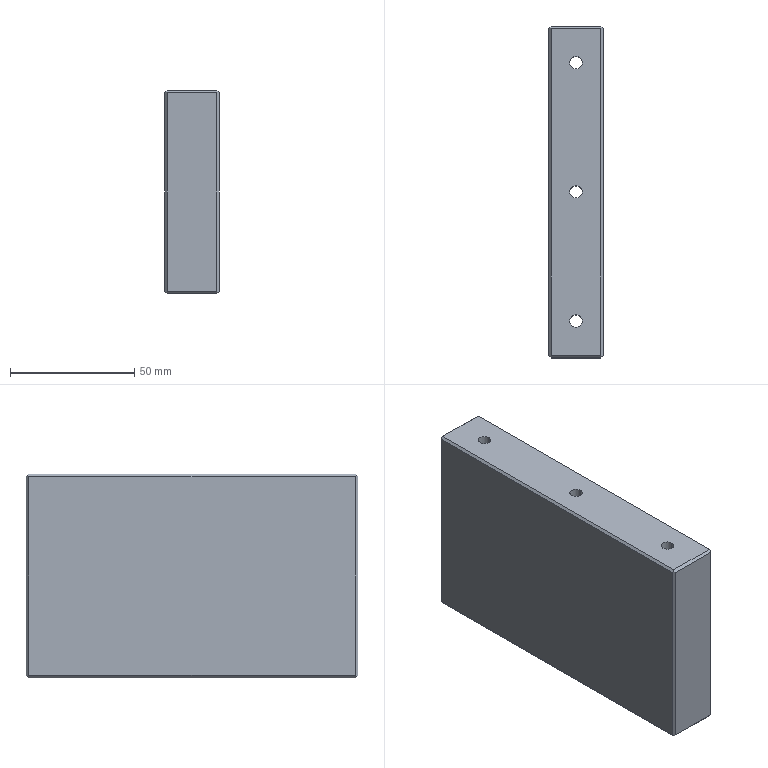Part | Creo | features DATUM PLANE 3, CHAMFER 1, COORDINATE SYSTEM 1, CURVE 1, PROTRUSION 1 | 1 solid | 24 faces | box 22 x 133.5 x 82 mm | volume 235535 mm3 | plane 18 | cylinder 6 | commonest cylinder face diameters 5 x6
STEP:
#1=CARTESIAN_POINT('',(0.,0.,0.));
#2=DIRECTION('',(0.,0.,1.));
#3=DIRECTION('',(1.,0.,0.));
#4=AXIS2_PLACEMENT_3D('',#1,#2,#3);
#5=CARTESIAN_POINT('',(-10.,-65.75,0.));
#6=VERTEX_POINT('',#5);
#7=CARTESIAN_POINT('',(-10.,65.75,0.));
#8=VERTEX_POINT('',#7);
#9=CARTESIAN_POINT('',(-10.,-65.75,0.));
#10=DIRECTION('',(0.,1.,0.));
#11=VECTOR('',#10,131.5);
#12=LINE('',#9,#11);
#13=EDGE_CURVE('',#6,#8,#12,.T.);
#14=ORIENTED_EDGE('',*,*,#13,.F.);
#15=CARTESIAN_POINT('',(10.,-65.75,0.));
#16=VERTEX_POINT('',#15);
#17=CARTESIAN_POINT('',(10.,-65.75,0.));
#18=DIRECTION('',(-1.,0.,0.));
#19=VECTOR('',#18,20.);
#20=LINE('',#17,#19);
#21=EDGE_CURVE('',#16,#6,#20,.T.);
#22=ORIENTED_EDGE('',*,*,#21,.F.);
#23=CARTESIAN_POINT('',(10.,65.75,0.));
#24=VERTEX_POINT('',#23);
#25=CARTESIAN_POINT('',(10.,65.75,0.));
#26=DIRECTION('',(0.,-1.,0.));
#27=VECTOR('',#26,131.5);
#28=LINE('',#25,#27);
#29=EDGE_CURVE('',#24,#16,#28,.T.);
#30=ORIENTED_EDGE('',*,*,#29,.F.);
#31=CARTESIAN_POINT('',(-10.,65.75,0.));
#32=DIRECTION('',(1.,0.,0.));
#33=VECTOR('',#32,20.);
#34=LINE('',#31,#33);
#35=EDGE_CURVE('',#8,#24,#34,.T.);
#36=ORIENTED_EDGE('',*,*,#35,.F.);
#37=EDGE_LOOP('',(#14,#22,#30,#36));
#38=FACE_OUTER_BOUND('',#37,.F.);
#39=CARTESIAN_POINT('',(2.5,0.,0.));
#40=VERTEX_POINT('',#39);
#41=CARTESIAN_POINT('',(-2.5,0.,0.));
#42=VERTEX_POINT('',#41);
#43=CARTESIAN_POINT('',(0.,0.,0.));
#44=DIRECTION('',(0.,0.,-1.));
#45=DIRECTION('',(1.,0.,0.));
#46=AXIS2_PLACEMENT_3D('',#43,#44,#45);
#47=CIRCLE('',#46,2.5);
#48=EDGE_CURVE('',#40,#42,#47,.T.);
#49=ORIENTED_EDGE('',*,*,#48,.T.);
#50=CARTESIAN_POINT('',(0.,0.,0.));
#51=DIRECTION('',(0.,0.,-1.));
#52=DIRECTION('',(-1.,0.,0.));
#53=AXIS2_PLACEMENT_3D('',#50,#51,#52);
#54=CIRCLE('',#53,2.5);
#55=EDGE_CURVE('',#42,#40,#54,.T.);
#56=ORIENTED_EDGE('',*,*,#55,.T.);
#57=EDGE_LOOP('',(#49,#56));
#58=FACE_BOUND('',#57,.F.);
#59=CARTESIAN_POINT('',(2.5,-52.,0.));
#60=VERTEX_POINT('',#59);
#61=CARTESIAN_POINT('',(-2.5,-52.,0.));
#62=VERTEX_POINT('',#61);
#63=CARTESIAN_POINT('',(0.,-52.,0.));
#64=DIRECTION('',(0.,0.,-1.));
#65=DIRECTION('',(1.,0.,0.));
#66=AXIS2_PLACEMENT_3D('',#63,#64,#65);
#67=CIRCLE('',#66,2.5);
#68=EDGE_CURVE('',#60,#62,#67,.T.);
#69=ORIENTED_EDGE('',*,*,#68,.T.);
#70=CARTESIAN_POINT('',(0.,-52.,0.));
#71=DIRECTION('',(0.,0.,-1.));
#72=DIRECTION('',(-1.,0.,0.));
#73=AXIS2_PLACEMENT_3D('',#70,#71,#72);
#74=CIRCLE('',#73,2.5);
#75=EDGE_CURVE('',#62,#60,#74,.T.);
#76=ORIENTED_EDGE('',*,*,#75,.T.);
#77=EDGE_LOOP('',(#69,#76));
#78=FACE_BOUND('',#77,.F.);
#79=CARTESIAN_POINT('',(2.5,52.,0.));
#80=VERTEX_POINT('',#79);
#81=CARTESIAN_POINT('',(-2.5,52.,0.));
#82=VERTEX_POINT('',#81);
#83=CARTESIAN_POINT('',(0.,52.,0.));
#84=DIRECTION('',(0.,0.,-1.));
#85=DIRECTION('',(1.,0.,0.));
#86=AXIS2_PLACEMENT_3D('',#83,#84,#85);
#87=CIRCLE('',#86,2.5);
#88=EDGE_CURVE('',#80,#82,#87,.T.);
#89=ORIENTED_EDGE('',*,*,#88,.T.);
#90=CARTESIAN_POINT('',(0.,52.,0.));
#91=DIRECTION('',(0.,0.,-1.));
#92=DIRECTION('',(-1.,0.,0.));
#93=AXIS2_PLACEMENT_3D('',#90,#91,#92);
#94=CIRCLE('',#93,2.5);
#95=EDGE_CURVE('',#82,#80,#94,.T.);
#96=ORIENTED_EDGE('',*,*,#95,.T.);
#97=EDGE_LOOP('',(#89,#96));
#98=FACE_BOUND('',#97,.F.);
#99=CARTESIAN_POINT('',(0.,0.,0.));
#100=DIRECTION('',(0.,0.,1.));
#101=DIRECTION('',(1.,0.,0.));
#102=AXIS2_PLACEMENT_3D('',#99,#100,#101);
#103=PLANE('',#102);
#104=ADVANCED_FACE('',(#38,#58,#78,#98),#103,.F.);
#105=ORIENTED_EDGE('',*,*,#88,.F.);
#106=CARTESIAN_POINT('',(2.5,52.,82.));
#107=VERTEX_POINT('',#106);
#108=CARTESIAN_POINT('',(2.5,52.,0.));
#109=DIRECTION('',(0.,0.,1.));
#110=VECTOR('',#109,82.);
#111=LINE('',#108,#110);
#112=EDGE_CURVE('',#80,#107,#111,.T.);
#113=ORIENTED_EDGE('',*,*,#112,.T.);
#114=CARTESIAN_POINT('',(-2.5,52.,82.));
#115=VERTEX_POINT('',#114);
#116=CARTESIAN_POINT('',(0.,52.,82.));
#117=DIRECTION('',(0.,0.,-1.));
#118=DIRECTION('',(1.,0.,0.));
#119=AXIS2_PLACEMENT_3D('',#116,#117,#118);
#120=CIRCLE('',#119,2.5);
#121=EDGE_CURVE('',#107,#115,#120,.T.);
#122=ORIENTED_EDGE('',*,*,#121,.T.);
#123=CARTESIAN_POINT('',(-2.5,52.,0.));
#124=DIRECTION('',(0.,0.,1.));
#125=VECTOR('',#124,82.);
#126=LINE('',#123,#125);
#127=EDGE_CURVE('',#82,#115,#126,.T.);
#128=ORIENTED_EDGE('',*,*,#127,.F.);
#129=EDGE_LOOP('',(#105,#113,#122,#128));
#130=FACE_OUTER_BOUND('',#129,.F.);
#131=CARTESIAN_POINT('',(0.,52.,0.));
#132=DIRECTION('',(0.,0.,1.));
#133=DIRECTION('',(1.,0.,0.));
#134=AXIS2_PLACEMENT_3D('',#131,#132,#133);
#135=CYLINDRICAL_SURFACE('',#134,2.5);
#136=ADVANCED_FACE('',(#130),#135,.F.);
#137=ORIENTED_EDGE('',*,*,#95,.F.);
#138=ORIENTED_EDGE('',*,*,#127,.T.);
#139=CARTESIAN_POINT('',(0.,52.,82.));
#140=DIRECTION('',(0.,0.,-1.));
#141=DIRECTION('',(-1.,0.,0.));
#142=AXIS2_PLACEMENT_3D('',#139,#140,#141);
#143=CIRCLE('',#142,2.5);
#144=EDGE_CURVE('',#115,#107,#143,.T.);
#145=ORIENTED_EDGE('',*,*,#144,.T.);
#146=ORIENTED_EDGE('',*,*,#112,.F.);
#147=EDGE_LOOP('',(#137,#138,#145,#146));
#148=FACE_OUTER_BOUND('',#147,.F.);
#149=CARTESIAN_POINT('',(0.,52.,0.));
#150=DIRECTION('',(0.,0.,1.));
#151=DIRECTION('',(1.,0.,0.));
#152=AXIS2_PLACEMENT_3D('',#149,#150,#151);
#153=CYLINDRICAL_SURFACE('',#152,2.5);
#154=ADVANCED_FACE('',(#148),#153,.F.);
#155=CARTESIAN_POINT('',(10.,65.75,82.));
#156=VERTEX_POINT('',#155);
#157=CARTESIAN_POINT('',(-10.,65.75,82.));
#158=VERTEX_POINT('',#157);
#159=CARTESIAN_POINT('',(10.,65.75,82.));
#160=DIRECTION('',(-1.,0.,0.));
#161=VECTOR('',#160,20.);
#162=LINE('',#159,#161);
#163=EDGE_CURVE('',#156,#158,#162,.T.);
#164=ORIENTED_EDGE('',*,*,#163,.F.);
#165=CARTESIAN_POINT('',(10.,-65.75,82.));
#166=VERTEX_POINT('',#165);
#167=CARTESIAN_POINT('',(10.,-65.75,82.));
#168=DIRECTION('',(0.,1.,0.));
#169=VECTOR('',#168,131.5);
#170=LINE('',#167,#169);
#171=EDGE_CURVE('',#166,#156,#170,.T.);
#172=ORIENTED_EDGE('',*,*,#171,.F.);
#173=CARTESIAN_POINT('',(-10.,-65.75,82.));
#174=VERTEX_POINT('',#173);
#175=CARTESIAN_POINT('',(-10.,-65.75,82.));
#176=DIRECTION('',(1.,0.,0.));
#177=VECTOR('',#176,20.);
#178=LINE('',#175,#177);
#179=EDGE_CURVE('',#174,#166,#178,.T.);
#180=ORIENTED_EDGE('',*,*,#179,.F.);
#181=CARTESIAN_POINT('',(-10.,65.75,82.));
#182=DIRECTION('',(0.,-1.,0.));
#183=VECTOR('',#182,131.5);
#184=LINE('',#181,#183);
#185=EDGE_CURVE('',#158,#174,#184,.T.);
#186=ORIENTED_EDGE('',*,*,#185,.F.);
#187=EDGE_LOOP('',(#164,#172,#180,#186));
#188=FACE_OUTER_BOUND('',#187,.F.);
#189=CARTESIAN_POINT('',(2.5,0.,82.));
#190=VERTEX_POINT('',#189);
#191=CARTESIAN_POINT('',(-2.5,0.,82.));
#192=VERTEX_POINT('',#191);
#193=CARTESIAN_POINT('',(0.,0.,82.));
#194=DIRECTION('',(0.,0.,-1.));
#195=DIRECTION('',(1.,0.,0.));
#196=AXIS2_PLACEMENT_3D('',#193,#194,#195);
#197=CIRCLE('',#196,2.5);
#198=EDGE_CURVE('',#190,#192,#197,.T.);
#199=ORIENTED_EDGE('',*,*,#198,.F.);
#200=CARTESIAN_POINT('',(0.,0.,82.));
#201=DIRECTION('',(0.,0.,-1.));
#202=DIRECTION('',(-1.,0.,0.));
#203=AXIS2_PLACEMENT_3D('',#200,#201,#202);
#204=CIRCLE('',#203,2.5);
#205=EDGE_CURVE('',#192,#190,#204,.T.);
#206=ORIENTED_EDGE('',*,*,#205,.F.);
#207=EDGE_LOOP('',(#199,#206));
#208=FACE_BOUND('',#207,.F.);
#209=CARTESIAN_POINT('',(2.5,-52.,82.));
#210=VERTEX_POINT('',#209);
#211=CARTESIAN_POINT('',(-2.5,-52.,82.));
#212=VERTEX_POINT('',#211);
#213=CARTESIAN_POINT('',(0.,-52.,82.));
#214=DIRECTION('',(0.,0.,-1.));
#215=DIRECTION('',(1.,0.,0.));
#216=AXIS2_PLACEMENT_3D('',#213,#214,#215);
#217=CIRCLE('',#216,2.5);
#218=EDGE_CURVE('',#210,#212,#217,.T.);
#219=ORIENTED_EDGE('',*,*,#218,.F.);
#220=CARTESIAN_POINT('',(0.,-52.,82.));
#221=DIRECTION('',(0.,0.,-1.));
#222=DIRECTION('',(-1.,0.,0.));
#223=AXIS2_PLACEMENT_3D('',#220,#221,#222);
#224=CIRCLE('',#223,2.5);
#225=EDGE_CURVE('',#212,#210,#224,.T.);
#226=ORIENTED_EDGE('',*,*,#225,.F.);
#227=EDGE_LOOP('',(#219,#226));
#228=FACE_BOUND('',#227,.F.);
#229=ORIENTED_EDGE('',*,*,#121,.F.);
#230=ORIENTED_EDGE('',*,*,#144,.F.);
#231=EDGE_LOOP('',(#229,#230));
#232=FACE_BOUND('',#231,.F.);
#233=CARTESIAN_POINT('',(0.,0.,82.));
#234=DIRECTION('',(0.,0.,1.));
#235=DIRECTION('',(1.,0.,0.));
#236=AXIS2_PLACEMENT_3D('',#233,#234,#235);
#237=PLANE('',#236);
#238=ADVANCED_FACE('',(#188,#208,#228,#232),#237,.T.);
#239=ORIENTED_EDGE('',*,*,#48,.F.);
#240=CARTESIAN_POINT('',(2.5,0.,0.));
#241=DIRECTION('',(0.,0.,1.));
#242=VECTOR('',#241,82.);
#243=LINE('',#240,#242);
#244=EDGE_CURVE('',#40,#190,#243,.T.);
#245=ORIENTED_EDGE('',*,*,#244,.T.);
#246=ORIENTED_EDGE('',*,*,#198,.T.);
#247=CARTESIAN_POINT('',(-2.5,0.,0.));
#248=DIRECTION('',(0.,0.,1.));
#249=VECTOR('',#248,82.);
#250=LINE('',#247,#249);
#251=EDGE_CURVE('',#42,#192,#250,.T.);
#252=ORIENTED_EDGE('',*,*,#251,.F.);
#253=EDGE_LOOP('',(#239,#245,#246,#252));
#254=FACE_OUTER_BOUND('',#253,.F.);
#255=CARTESIAN_POINT('',(0.,0.,0.));
#256=DIRECTION('',(0.,0.,1.));
#257=DIRECTION('',(1.,0.,0.));
#258=AXIS2_PLACEMENT_3D('',#255,#256,#257);
#259=CYLINDRICAL_SURFACE('',#258,2.5);
#260=ADVANCED_FACE('',(#254),#259,.F.);
#261=ORIENTED_EDGE('',*,*,#55,.F.);
#262=ORIENTED_EDGE('',*,*,#251,.T.);
#263=ORIENTED_EDGE('',*,*,#205,.T.);
#264=ORIENTED_EDGE('',*,*,#244,.F.);
#265=EDGE_LOOP('',(#261,#262,#263,#264));
#266=FACE_OUTER_BOUND('',#265,.F.);
#267=CARTESIAN_POINT('',(0.,0.,0.));
#268=DIRECTION('',(0.,0.,1.));
#269=DIRECTION('',(1.,0.,0.));
#270=AXIS2_PLACEMENT_3D('',#267,#268,#269);
#271=CYLINDRICAL_SURFACE('',#270,2.5);
#272=ADVANCED_FACE('',(#266),#271,.F.);
#273=ORIENTED_EDGE('',*,*,#68,.F.);
#274=CARTESIAN_POINT('',(2.5,-52.,0.));
#275=DIRECTION('',(0.,0.,1.));
#276=VECTOR('',#275,82.);
#277=LINE('',#274,#276);
#278=EDGE_CURVE('',#60,#210,#277,.T.);
#279=ORIENTED_EDGE('',*,*,#278,.T.);
#280=ORIENTED_EDGE('',*,*,#218,.T.);
#281=CARTESIAN_POINT('',(-2.5,-52.,0.));
#282=DIRECTION('',(0.,0.,1.));
#283=VECTOR('',#282,82.);
#284=LINE('',#281,#283);
#285=EDGE_CURVE('',#62,#212,#284,.T.);
#286=ORIENTED_EDGE('',*,*,#285,.F.);
#287=EDGE_LOOP('',(#273,#279,#280,#286));
#288=FACE_OUTER_BOUND('',#287,.F.);
#289=CARTESIAN_POINT('',(0.,-52.,0.));
#290=DIRECTION('',(0.,0.,1.));
#291=DIRECTION('',(1.,0.,0.));
#292=AXIS2_PLACEMENT_3D('',#289,#290,#291);
#293=CYLINDRICAL_SURFACE('',#292,2.5);
#294=ADVANCED_FACE('',(#288),#293,.F.);
#295=ORIENTED_EDGE('',*,*,#75,.F.);
#296=ORIENTED_EDGE('',*,*,#285,.T.);
#297=ORIENTED_EDGE('',*,*,#225,.T.);
#298=ORIENTED_EDGE('',*,*,#278,.F.);
#299=EDGE_LOOP('',(#295,#296,#297,#298));
#300=FACE_OUTER_BOUND('',#299,.F.);
#301=CARTESIAN_POINT('',(0.,-52.,0.));
#302=DIRECTION('',(0.,0.,1.));
#303=DIRECTION('',(1.,0.,0.));
#304=AXIS2_PLACEMENT_3D('',#301,#302,#303);
#305=CYLINDRICAL_SURFACE('',#304,2.5);
#306=ADVANCED_FACE('',(#300),#305,.F.);
#307=CARTESIAN_POINT('',(10.,66.75,81.));
#308=VERTEX_POINT('',#307);
#309=CARTESIAN_POINT('',(-10.,66.75,81.));
#310=VERTEX_POINT('',#309);
#311=CARTESIAN_POINT('',(10.,66.75,81.));
#312=DIRECTION('',(-1.,0.,0.));
#313=VECTOR('',#312,20.);
#314=LINE('',#311,#313);
#315=EDGE_CURVE('',#308,#310,#314,.T.);
#316=ORIENTED_EDGE('',*,*,#315,.F.);
#317=CARTESIAN_POINT('',(10.5,66.25,81.5));
#318=VERTEX_POINT('',#317);
#319=CARTESIAN_POINT('',(10.,66.75,81.));
#320=DIRECTION('',(0.5774,-0.5774,0.5774));
#321=VECTOR('',#320,0.866);
#322=LINE('',#319,#321);
#323=EDGE_CURVE('',#308,#318,#322,.T.);
#324=ORIENTED_EDGE('',*,*,#323,.T.);
#325=CARTESIAN_POINT('',(10.,65.75,82.));
#326=DIRECTION('',(0.5774,0.5774,-0.5774));
#327=VECTOR('',#326,0.866);
#328=LINE('',#325,#327);
#329=EDGE_CURVE('',#156,#318,#328,.T.);
#330=ORIENTED_EDGE('',*,*,#329,.F.);
#331=ORIENTED_EDGE('',*,*,#163,.T.);
#332=CARTESIAN_POINT('',(-10.5,66.25,81.5));
#333=VERTEX_POINT('',#332);
#334=CARTESIAN_POINT('',(-10.,65.75,82.));
#335=DIRECTION('',(-0.5774,0.5774,-0.5774));
#336=VECTOR('',#335,0.866);
#337=LINE('',#334,#336);
#338=EDGE_CURVE('',#158,#333,#337,.T.);
#339=ORIENTED_EDGE('',*,*,#338,.T.);
#340=CARTESIAN_POINT('',(-10.5,66.25,81.5));
#341=DIRECTION('',(0.5774,0.5774,-0.5774));
#342=VECTOR('',#341,0.866);
#343=LINE('',#340,#342);
#344=EDGE_CURVE('',#333,#310,#343,.T.);
#345=ORIENTED_EDGE('',*,*,#344,.T.);
#346=EDGE_LOOP('',(#316,#324,#330,#331,#339,#345));
#347=FACE_OUTER_BOUND('',#346,.F.);
#348=CARTESIAN_POINT('',(0.,66.25,81.5));
#349=DIRECTION('',(0.,0.7071,0.7071));
#350=DIRECTION('',(0.,0.7071,-0.7071));
#351=AXIS2_PLACEMENT_3D('',#348,#349,#350);
#352=PLANE('',#351);
#353=ADVANCED_FACE('',(#347),#352,.T.);
#354=CARTESIAN_POINT('',(10.,66.75,1.));
#355=VERTEX_POINT('',#354);
#356=CARTESIAN_POINT('',(10.,66.75,81.));
#357=DIRECTION('',(0.,0.,-1.));
#358=VECTOR('',#357,80.);
#359=LINE('',#356,#358);
#360=EDGE_CURVE('',#308,#355,#359,.T.);
#361=ORIENTED_EDGE('',*,*,#360,.F.);
#362=ORIENTED_EDGE('',*,*,#315,.T.);
#363=CARTESIAN_POINT('',(-10.,66.75,1.));
#364=VERTEX_POINT('',#363);
#365=CARTESIAN_POINT('',(-10.,66.75,81.));
#366=DIRECTION('',(0.,0.,-1.));
#367=VECTOR('',#366,80.);
#368=LINE('',#365,#367);
#369=EDGE_CURVE('',#310,#364,#368,.T.);
#370=ORIENTED_EDGE('',*,*,#369,.T.);
#371=CARTESIAN_POINT('',(-10.,66.75,1.));
#372=DIRECTION('',(1.,0.,0.));
#373=VECTOR('',#372,20.);
#374=LINE('',#371,#373);
#375=EDGE_CURVE('',#364,#355,#374,.T.);
#376=ORIENTED_EDGE('',*,*,#375,.T.);
#377=EDGE_LOOP('',(#361,#362,#370,#376));
#378=FACE_OUTER_BOUND('',#377,.F.);
#379=CARTESIAN_POINT('',(11.,66.75,0.));
#380=DIRECTION('',(0.,1.,0.));
#381=DIRECTION('',(-1.,0.,0.));
#382=AXIS2_PLACEMENT_3D('',#379,#380,#381);
#383=PLANE('',#382);
#384=ADVANCED_FACE('',(#378),#383,.T.);
#385=ORIENTED_EDGE('',*,*,#360,.T.);
#386=CARTESIAN_POINT('',(10.5,66.25,0.5));
#387=VERTEX_POINT('',#386);
#388=CARTESIAN_POINT('',(10.,66.75,1.));
#389=DIRECTION('',(0.5774,-0.5774,-0.5774));
#390=VECTOR('',#389,0.866);
#391=LINE('',#388,#390);
#392=EDGE_CURVE('',#355,#387,#391,.T.);
#393=ORIENTED_EDGE('',*,*,#392,.T.);
#394=CARTESIAN_POINT('',(11.,65.75,1.));
#395=VERTEX_POINT('',#394);
#396=CARTESIAN_POINT('',(11.,65.75,1.));
#397=DIRECTION('',(-0.5774,0.5774,-0.5774));
#398=VECTOR('',#397,0.866);
#399=LINE('',#396,#398);
#400=EDGE_CURVE('',#395,#387,#399,.T.);
#401=ORIENTED_EDGE('',*,*,#400,.F.);
#402=CARTESIAN_POINT('',(11.,65.75,81.));
#403=VERTEX_POINT('',#402);
#404=CARTESIAN_POINT('',(11.,65.75,81.));
#405=DIRECTION('',(0.,0.,-1.));
#406=VECTOR('',#405,80.);
#407=LINE('',#404,#406);
#408=EDGE_CURVE('',#403,#395,#407,.T.);
#409=ORIENTED_EDGE('',*,*,#408,.F.);
#410=CARTESIAN_POINT('',(10.5,66.25,81.5));
#411=DIRECTION('',(0.5774,-0.5774,-0.5774));
#412=VECTOR('',#411,0.866);
#413=LINE('',#410,#412);
#414=EDGE_CURVE('',#318,#403,#413,.T.);
#415=ORIENTED_EDGE('',*,*,#414,.F.);
#416=ORIENTED_EDGE('',*,*,#323,.F.);
#417=EDGE_LOOP('',(#385,#393,#401,#409,#415,#416));
#418=FACE_OUTER_BOUND('',#417,.F.);
#419=CARTESIAN_POINT('',(10.5,66.25,41.));
#420=DIRECTION('',(0.7071,0.7071,0.));
#421=DIRECTION('',(0.7071,-0.7071,0.));
#422=AXIS2_PLACEMENT_3D('',#419,#420,#421);
#423=PLANE('',#422);
#424=ADVANCED_FACE('',(#418),#423,.T.);
#425=ORIENTED_EDGE('',*,*,#35,.T.);
#426=CARTESIAN_POINT('',(10.5,66.25,0.5));
#427=DIRECTION('',(-0.5774,-0.5774,-0.5774));
#428=VECTOR('',#427,0.866);
#429=LINE('',#426,#428);
#430=EDGE_CURVE('',#387,#24,#429,.T.);
#431=ORIENTED_EDGE('',*,*,#430,.F.);
#432=ORIENTED_EDGE('',*,*,#392,.F.);
#433=ORIENTED_EDGE('',*,*,#375,.F.);
#434=CARTESIAN_POINT('',(-10.5,66.25,0.5));
#435=VERTEX_POINT('',#434);
#436=CARTESIAN_POINT('',(-10.,66.75,1.));
#437=DIRECTION('',(-0.5774,-0.5774,-0.5774));
#438=VECTOR('',#437,0.866);
#439=LINE('',#436,#438);
#440=EDGE_CURVE('',#364,#435,#439,.T.);
#441=ORIENTED_EDGE('',*,*,#440,.T.);
#442=CARTESIAN_POINT('',(-10.5,66.25,0.5));
#443=DIRECTION('',(0.5774,-0.5774,-0.5774));
#444=VECTOR('',#443,0.866);
#445=LINE('',#442,#444);
#446=EDGE_CURVE('',#435,#8,#445,.T.);
#447=ORIENTED_EDGE('',*,*,#446,.T.);
#448=EDGE_LOOP('',(#425,#431,#432,#433,#441,#447));
#449=FACE_OUTER_BOUND('',#448,.F.);
#450=CARTESIAN_POINT('',(0.,66.25,0.5));
#451=DIRECTION('',(0.,0.7071,-0.7071));
#452=DIRECTION('',(0.,0.7071,0.7071));
#453=AXIS2_PLACEMENT_3D('',#450,#451,#452);
#454=PLANE('',#453);
#455=ADVANCED_FACE('',(#449),#454,.T.);
#456=CARTESIAN_POINT('',(11.,-65.75,1.));
#457=VERTEX_POINT('',#456);
#458=CARTESIAN_POINT('',(11.,65.75,1.));
#459=DIRECTION('',(0.,-1.,0.));
#460=VECTOR('',#459,131.5);
#461=LINE('',#458,#460);
#462=EDGE_CURVE('',#395,#457,#461,.T.);
#463=ORIENTED_EDGE('',*,*,#462,.F.);
#464=ORIENTED_EDGE('',*,*,#400,.T.);
#465=ORIENTED_EDGE('',*,*,#430,.T.);
#466=ORIENTED_EDGE('',*,*,#29,.T.);
#467=CARTESIAN_POINT('',(10.5,-66.25,0.5));
#468=VERTEX_POINT('',#467);
#469=CARTESIAN_POINT('',(10.,-65.75,0.));
#470=DIRECTION('',(0.5774,-0.5774,0.5774));
#471=VECTOR('',#470,0.866);
#472=LINE('',#469,#471);
#473=EDGE_CURVE('',#16,#468,#472,.T.);
#474=ORIENTED_EDGE('',*,*,#473,.T.);
#475=CARTESIAN_POINT('',(10.5,-66.25,0.5));
#476=DIRECTION('',(0.5774,0.5774,0.5774));
#477=VECTOR('',#476,0.866);
#478=LINE('',#475,#477);
#479=EDGE_CURVE('',#468,#457,#478,.T.);
#480=ORIENTED_EDGE('',*,*,#479,.T.);
#481=EDGE_LOOP('',(#463,#464,#465,#466,#474,#480));
#482=FACE_OUTER_BOUND('',#481,.F.);
#483=CARTESIAN_POINT('',(10.5,0.,0.5));
#484=DIRECTION('',(0.7071,0.,-0.7071));
#485=DIRECTION('',(0.7071,0.,0.7071));
#486=AXIS2_PLACEMENT_3D('',#483,#484,#485);
#487=PLANE('',#486);
#488=ADVANCED_FACE('',(#482),#487,.T.);
#489=ORIENTED_EDGE('',*,*,#408,.T.);
#490=ORIENTED_EDGE('',*,*,#462,.T.);
#491=CARTESIAN_POINT('',(11.,-65.75,81.));
#492=VERTEX_POINT('',#491);
#493=CARTESIAN_POINT('',(11.,-65.75,81.));
#494=DIRECTION('',(0.,0.,-1.));
#495=VECTOR('',#494,80.);
#496=LINE('',#493,#495);
#497=EDGE_CURVE('',#492,#457,#496,.T.);
#498=ORIENTED_EDGE('',*,*,#497,.F.);
#499=CARTESIAN_POINT('',(11.,-65.75,81.));
#500=DIRECTION('',(0.,1.,0.));
#501=VECTOR('',#500,131.5);
#502=LINE('',#499,#501);
#503=EDGE_CURVE('',#492,#403,#502,.T.);
#504=ORIENTED_EDGE('',*,*,#503,.T.);
#505=EDGE_LOOP('',(#489,#490,#498,#504));
#506=FACE_OUTER_BOUND('',#505,.F.);
#507=CARTESIAN_POINT('',(11.,-66.75,0.));
#508=DIRECTION('',(1.,0.,0.));
#509=DIRECTION('',(0.,1.,0.));
#510=AXIS2_PLACEMENT_3D('',#507,#508,#509);
#511=PLANE('',#510);
#512=ADVANCED_FACE('',(#506),#511,.T.);
#513=ORIENTED_EDGE('',*,*,#497,.T.);
#514=ORIENTED_EDGE('',*,*,#479,.F.);
#515=CARTESIAN_POINT('',(10.,-66.75,1.));
#516=VERTEX_POINT('',#515);
#517=CARTESIAN_POINT('',(10.,-66.75,1.));
#518=DIRECTION('',(0.5774,0.5774,-0.5774));
#519=VECTOR('',#518,0.866);
#520=LINE('',#517,#519);
#521=EDGE_CURVE('',#516,#468,#520,.T.);
#522=ORIENTED_EDGE('',*,*,#521,.F.);
#523=CARTESIAN_POINT('',(10.,-66.75,81.));
#524=VERTEX_POINT('',#523);
#525=CARTESIAN_POINT('',(10.,-66.75,81.));
#526=DIRECTION('',(0.,0.,-1.));
#527=VECTOR('',#526,80.);
#528=LINE('',#525,#527);
#529=EDGE_CURVE('',#524,#516,#528,.T.);
#530=ORIENTED_EDGE('',*,*,#529,.F.);
#531=CARTESIAN_POINT('',(10.5,-66.25,81.5));
#532=VERTEX_POINT('',#531);
#533=CARTESIAN_POINT('',(10.,-66.75,81.));
#534=DIRECTION('',(0.5774,0.5774,0.5774));
#535=VECTOR('',#534,0.866);
#536=LINE('',#533,#535);
#537=EDGE_CURVE('',#524,#532,#536,.T.);
#538=ORIENTED_EDGE('',*,*,#537,.T.);
#539=CARTESIAN_POINT('',(11.,-65.75,81.));
#540=DIRECTION('',(-0.5774,-0.5774,0.5774));
#541=VECTOR('',#540,0.866);
#542=LINE('',#539,#541);
#543=EDGE_CURVE('',#492,#532,#542,.T.);
#544=ORIENTED_EDGE('',*,*,#543,.F.);
#545=EDGE_LOOP('',(#513,#514,#522,#530,#538,#544));
#546=FACE_OUTER_BOUND('',#545,.F.);
#547=CARTESIAN_POINT('',(10.5,-66.25,41.));
#548=DIRECTION('',(0.7071,-0.7071,0.));
#549=DIRECTION('',(-0.7071,-0.7071,0.));
#550=AXIS2_PLACEMENT_3D('',#547,#548,#549);
#551=PLANE('',#550);
#552=ADVANCED_FACE('',(#546),#551,.T.);
#553=CARTESIAN_POINT('',(-10.,-66.75,1.));
#554=VERTEX_POINT('',#553);
#555=CARTESIAN_POINT('',(10.,-66.75,1.));
#556=DIRECTION('',(-1.,0.,0.));
#557=VECTOR('',#556,20.);
#558=LINE('',#555,#557);
#559=EDGE_CURVE('',#516,#554,#558,.T.);
#560=ORIENTED_EDGE('',*,*,#559,.F.);
#561=ORIENTED_EDGE('',*,*,#521,.T.);
#562=ORIENTED_EDGE('',*,*,#473,.F.);
#563=ORIENTED_EDGE('',*,*,#21,.T.);
#564=CARTESIAN_POINT('',(-10.5,-66.25,0.5));
#565=VERTEX_POINT('',#564);
#566=CARTESIAN_POINT('',(-10.5,-66.25,0.5));
#567=DIRECTION('',(0.5774,0.5774,-0.5774));
#568=VECTOR('',#567,0.866);
#569=LINE('',#566,#568);
#570=EDGE_CURVE('',#565,#6,#569,.T.);
#571=ORIENTED_EDGE('',*,*,#570,.F.);
#572=CARTESIAN_POINT('',(-10.,-66.75,1.));
#573=DIRECTION('',(-0.5774,0.5774,-0.5774));
#574=VECTOR('',#573,0.866);
#575=LINE('',#572,#574);
#576=EDGE_CURVE('',#554,#565,#575,.T.);
#577=ORIENTED_EDGE('',*,*,#576,.F.);
#578=EDGE_LOOP('',(#560,#561,#562,#563,#571,#577));
#579=FACE_OUTER_BOUND('',#578,.F.);
#580=CARTESIAN_POINT('',(0.,-66.25,0.5));
#581=DIRECTION('',(0.,-0.7071,-0.7071));
#582=DIRECTION('',(0.,-0.7071,0.7071));
#583=AXIS2_PLACEMENT_3D('',#580,#581,#582);
#584=PLANE('',#583);
#585=ADVANCED_FACE('',(#579),#584,.T.);
#586=ORIENTED_EDGE('',*,*,#529,.T.);
#587=ORIENTED_EDGE('',*,*,#559,.T.);
#588=CARTESIAN_POINT('',(-10.,-66.75,81.));
#589=VERTEX_POINT('',#588);
#590=CARTESIAN_POINT('',(-10.,-66.75,81.));
#591=DIRECTION('',(0.,0.,-1.));
#592=VECTOR('',#591,80.);
#593=LINE('',#590,#592);
#594=EDGE_CURVE('',#589,#554,#593,.T.);
#595=ORIENTED_EDGE('',*,*,#594,.F.);
#596=CARTESIAN_POINT('',(-10.,-66.75,81.));
#597=DIRECTION('',(1.,0.,0.));
#598=VECTOR('',#597,20.);
#599=LINE('',#596,#598);
#600=EDGE_CURVE('',#589,#524,#599,.T.);
#601=ORIENTED_EDGE('',*,*,#600,.T.);
#602=EDGE_LOOP('',(#586,#587,#595,#601));
#603=FACE_OUTER_BOUND('',#602,.F.);
#604=CARTESIAN_POINT('',(-11.,-66.75,0.));
#605=DIRECTION('',(0.,-1.,0.));
#606=DIRECTION('',(1.,0.,0.));
#607=AXIS2_PLACEMENT_3D('',#604,#605,#606);
#608=PLANE('',#607);
#609=ADVANCED_FACE('',(#603),#608,.T.);
#610=ORIENTED_EDGE('',*,*,#594,.T.);
#611=ORIENTED_EDGE('',*,*,#576,.T.);
#612=CARTESIAN_POINT('',(-11.,-65.75,1.));
#613=VERTEX_POINT('',#612);
#614=CARTESIAN_POINT('',(-11.,-65.75,1.));
#615=DIRECTION('',(0.5774,-0.5774,-0.5774));
#616=VECTOR('',#615,0.866);
#617=LINE('',#614,#616);
#618=EDGE_CURVE('',#613,#565,#617,.T.);
#619=ORIENTED_EDGE('',*,*,#618,.F.);
#620=CARTESIAN_POINT('',(-11.,-65.75,81.));
#621=VERTEX_POINT('',#620);
#622=CARTESIAN_POINT('',(-11.,-65.75,81.));
#623=DIRECTION('',(0.,0.,-1.));
#624=VECTOR('',#623,80.);
#625=LINE('',#622,#624);
#626=EDGE_CURVE('',#621,#613,#625,.T.);
#627=ORIENTED_EDGE('',*,*,#626,.F.);
#628=CARTESIAN_POINT('',(-10.5,-66.25,81.5));
#629=VERTEX_POINT('',#628);
#630=CARTESIAN_POINT('',(-10.5,-66.25,81.5));
#631=DIRECTION('',(-0.5774,0.5774,-0.5774));
#632=VECTOR('',#631,0.866);
#633=LINE('',#630,#632);
#634=EDGE_CURVE('',#629,#621,#633,.T.);
#635=ORIENTED_EDGE('',*,*,#634,.F.);
#636=CARTESIAN_POINT('',(-10.,-66.75,81.));
#637=DIRECTION('',(-0.5774,0.5774,0.5774));
#638=VECTOR('',#637,0.866);
#639=LINE('',#636,#638);
#640=EDGE_CURVE('',#589,#629,#639,.T.);
#641=ORIENTED_EDGE('',*,*,#640,.F.);
#642=EDGE_LOOP('',(#610,#611,#619,#627,#635,#641));
#643=FACE_OUTER_BOUND('',#642,.F.);
#644=CARTESIAN_POINT('',(-10.5,-66.25,41.));
#645=DIRECTION('',(-0.7071,-0.7071,0.));
#646=DIRECTION('',(-0.7071,0.7071,0.));
#647=AXIS2_PLACEMENT_3D('',#644,#645,#646);
#648=PLANE('',#647);
#649=ADVANCED_FACE('',(#643),#648,.T.);
#650=ORIENTED_EDGE('',*,*,#13,.T.);
#651=ORIENTED_EDGE('',*,*,#446,.F.);
#652=CARTESIAN_POINT('',(-11.,65.75,1.));
#653=VERTEX_POINT('',#652);
#654=CARTESIAN_POINT('',(-11.,65.75,1.));
#655=DIRECTION('',(0.5774,0.5774,-0.5774));
#656=VECTOR('',#655,0.866);
#657=LINE('',#654,#656);
#658=EDGE_CURVE('',#653,#435,#657,.T.);
#659=ORIENTED_EDGE('',*,*,#658,.F.);
#660=CARTESIAN_POINT('',(-11.,-65.75,1.));
#661=DIRECTION('',(0.,1.,0.));
#662=VECTOR('',#661,131.5);
#663=LINE('',#660,#662);
#664=EDGE_CURVE('',#613,#653,#663,.T.);
#665=ORIENTED_EDGE('',*,*,#664,.F.);
#666=ORIENTED_EDGE('',*,*,#618,.T.);
#667=ORIENTED_EDGE('',*,*,#570,.T.);
#668=EDGE_LOOP('',(#650,#651,#659,#665,#666,#667));
#669=FACE_OUTER_BOUND('',#668,.F.);
#670=CARTESIAN_POINT('',(-10.5,0.,0.5));
#671=DIRECTION('',(-0.7071,0.,-0.7071));
#672=DIRECTION('',(-0.7071,0.,0.7071));
#673=AXIS2_PLACEMENT_3D('',#670,#671,#672);
#674=PLANE('',#673);
#675=ADVANCED_FACE('',(#669),#674,.T.);
#676=CARTESIAN_POINT('',(-11.,65.75,81.));
#677=VERTEX_POINT('',#676);
#678=CARTESIAN_POINT('',(-11.,65.75,81.));
#679=DIRECTION('',(0.,0.,-1.));
#680=VECTOR('',#679,80.);
#681=LINE('',#678,#680);
#682=EDGE_CURVE('',#677,#653,#681,.T.);
#683=ORIENTED_EDGE('',*,*,#682,.T.);
#684=ORIENTED_EDGE('',*,*,#658,.T.);
#685=ORIENTED_EDGE('',*,*,#440,.F.);
#686=ORIENTED_EDGE('',*,*,#369,.F.);
#687=ORIENTED_EDGE('',*,*,#344,.F.);
#688=CARTESIAN_POINT('',(-11.,65.75,81.));
#689=DIRECTION('',(0.5774,0.5774,0.5774));
#690=VECTOR('',#689,0.866);
#691=LINE('',#688,#690);
#692=EDGE_CURVE('',#677,#333,#691,.T.);
#693=ORIENTED_EDGE('',*,*,#692,.F.);
#694=EDGE_LOOP('',(#683,#684,#685,#686,#687,#693));
#695=FACE_OUTER_BOUND('',#694,.F.);
#696=CARTESIAN_POINT('',(-10.5,66.25,41.));
#697=DIRECTION('',(-0.7071,0.7071,0.));
#698=DIRECTION('',(0.7071,0.7071,0.));
#699=AXIS2_PLACEMENT_3D('',#696,#697,#698);
#700=PLANE('',#699);
#701=ADVANCED_FACE('',(#695),#700,.T.);
#702=CARTESIAN_POINT('',(-11.,65.75,81.));
#703=DIRECTION('',(0.,-1.,0.));
#704=VECTOR('',#703,131.5);
#705=LINE('',#702,#704);
#706=EDGE_CURVE('',#677,#621,#705,.T.);
#707=ORIENTED_EDGE('',*,*,#706,.T.);
#708=ORIENTED_EDGE('',*,*,#626,.T.);
#709=ORIENTED_EDGE('',*,*,#664,.T.);
#710=ORIENTED_EDGE('',*,*,#682,.F.);
#711=EDGE_LOOP('',(#707,#708,#709,#710));
#712=FACE_OUTER_BOUND('',#711,.F.);
#713=CARTESIAN_POINT('',(-11.,66.75,0.));
#714=DIRECTION('',(-1.,0.,0.));
#715=DIRECTION('',(0.,-1.,0.));
#716=AXIS2_PLACEMENT_3D('',#713,#714,#715);
#717=PLANE('',#716);
#718=ADVANCED_FACE('',(#712),#717,.T.);
#719=ORIENTED_EDGE('',*,*,#706,.F.);
#720=ORIENTED_EDGE('',*,*,#692,.T.);
#721=ORIENTED_EDGE('',*,*,#338,.F.);
#722=ORIENTED_EDGE('',*,*,#185,.T.);
#723=CARTESIAN_POINT('',(-10.,-65.75,82.));
#724=DIRECTION('',(-0.5774,-0.5774,-0.5774));
#725=VECTOR('',#724,0.866);
#726=LINE('',#723,#725);
#727=EDGE_CURVE('',#174,#629,#726,.T.);
#728=ORIENTED_EDGE('',*,*,#727,.T.);
#729=ORIENTED_EDGE('',*,*,#634,.T.);
#730=EDGE_LOOP('',(#719,#720,#721,#722,#728,#729));
#731=FACE_OUTER_BOUND('',#730,.F.);
#732=CARTESIAN_POINT('',(-10.5,0.,81.5));
#733=DIRECTION('',(-0.7071,0.,0.7071));
#734=DIRECTION('',(-0.7071,0.,-0.7071));
#735=AXIS2_PLACEMENT_3D('',#732,#733,#734);
#736=PLANE('',#735);
#737=ADVANCED_FACE('',(#731),#736,.T.);
#738=ORIENTED_EDGE('',*,*,#179,.T.);
#739=CARTESIAN_POINT('',(10.5,-66.25,81.5));
#740=DIRECTION('',(-0.5774,0.5774,0.5774));
#741=VECTOR('',#740,0.866);
#742=LINE('',#739,#741);
#743=EDGE_CURVE('',#532,#166,#742,.T.);
#744=ORIENTED_EDGE('',*,*,#743,.F.);
#745=ORIENTED_EDGE('',*,*,#537,.F.);
#746=ORIENTED_EDGE('',*,*,#600,.F.);
#747=ORIENTED_EDGE('',*,*,#640,.T.);
#748=ORIENTED_EDGE('',*,*,#727,.F.);
#749=EDGE_LOOP('',(#738,#744,#745,#746,#747,#748));
#750=FACE_OUTER_BOUND('',#749,.F.);
#751=CARTESIAN_POINT('',(0.,-66.25,81.5));
#752=DIRECTION('',(0.,-0.7071,0.7071));
#753=DIRECTION('',(0.,-0.7071,-0.7071));
#754=AXIS2_PLACEMENT_3D('',#751,#752,#753);
#755=PLANE('',#754);
#756=ADVANCED_FACE('',(#750),#755,.T.);
#757=ORIENTED_EDGE('',*,*,#503,.F.);
#758=ORIENTED_EDGE('',*,*,#543,.T.);
#759=ORIENTED_EDGE('',*,*,#743,.T.);
#760=ORIENTED_EDGE('',*,*,#171,.T.);
#761=ORIENTED_EDGE('',*,*,#329,.T.);
#762=ORIENTED_EDGE('',*,*,#414,.T.);
#763=EDGE_LOOP('',(#757,#758,#759,#760,#761,#762));
#764=FACE_OUTER_BOUND('',#763,.F.);
#765=CARTESIAN_POINT('',(10.5,0.,81.5));
#766=DIRECTION('',(0.7071,0.,0.7071));
#767=DIRECTION('',(0.7071,0.,-0.7071));
#768=AXIS2_PLACEMENT_3D('',#765,#766,#767);
#769=PLANE('',#768);
#770=ADVANCED_FACE('',(#764),#769,.T.);
#771=CLOSED_SHELL('',(#104,#136,#154,#238,#260,#272,#294,#306,#353,#384,#424,#455,#488,#512,#552,#585,#609,#649,#675,#701,#718,#737,#756,#770));
#772=MANIFOLD_SOLID_BREP('',#771);
#773=(LENGTH_UNIT()NAMED_UNIT(*)SI_UNIT(.MILLI.,.METRE.));
#774=UNCERTAINTY_MEASURE_WITH_UNIT(LENGTH_MEASURE(0.01582),#773,'','');
#775=(NAMED_UNIT(*)PLANE_ANGLE_UNIT()SI_UNIT($,.RADIAN.));
#776=PLANE_ANGLE_MEASURE_WITH_UNIT(PLANE_ANGLE_MEASURE(0.01745),#775);
#777=(CONVERSION_BASED_UNIT('DEGREE',#776)NAMED_UNIT(*)PLANE_ANGLE_UNIT());
#778=(NAMED_UNIT(*)SI_UNIT($,.STERADIAN.)SOLID_ANGLE_UNIT());
#779=(GEOMETRIC_REPRESENTATION_CONTEXT(3)GLOBAL_UNCERTAINTY_ASSIGNED_CONTEXT((#774))GLOBAL_UNIT_ASSIGNED_CONTEXT((#773,#777,#778))REPRESENTATION_CONTEXT('',''));
#780=ADVANCED_BREP_SHAPE_REPRESENTATION('',(#4,#772),#779);